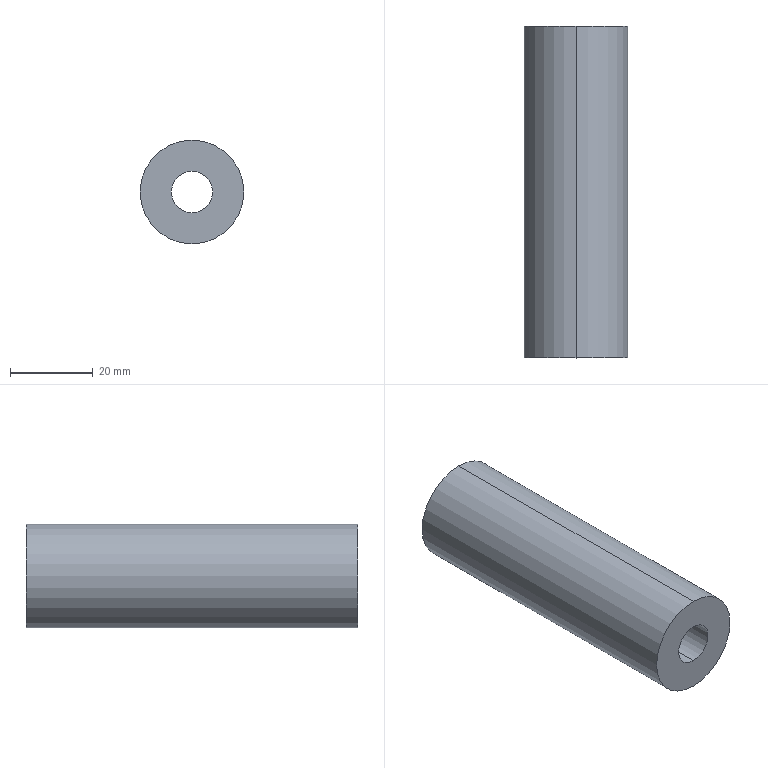Part | STEP file | 1 solid | 6 faces | box 25 x 80 x 25 mm | volume 32987 mm3 | cylinder 4 | plane 2 | commonest cylinder face diameters 10 x2 25 x2
STEP:
#1=CARTESIAN_POINT('',(0.,0.,0.));
#2=DIRECTION('',(0.,0.,1.));
#3=DIRECTION('',(1.,0.,0.));
#4=AXIS2_PLACEMENT_3D('',#1,#2,#3);
#5=CARTESIAN_POINT('',(0.,0.,12.5));
#6=VERTEX_POINT('',#5);
#7=CARTESIAN_POINT('',(0.,0.,-12.5));
#8=VERTEX_POINT('',#7);
#9=CARTESIAN_POINT('',(0.,0.,0.));
#10=DIRECTION('',(0.,1.,0.));
#11=DIRECTION('',(0.,0.,1.));
#12=AXIS2_PLACEMENT_3D('',#9,#10,#11);
#13=CIRCLE('',#12,12.5);
#14=CARTESIAN_POINT('',(0.,0.,0.));
#15=DIRECTION('',(0.,1.,0.));
#16=DIRECTION('',(0.,0.,1.));
#17=AXIS2_PLACEMENT_3D('',#14,#15,#16);
#18=CYLINDRICAL_SURFACE('',#17,12.5);
#19=CARTESIAN_POINT('',(0.,0.));
#20=DIRECTION('',(1.,0.));
#21=VECTOR('',#20,1.);
#22=LINE('',#19,#21);
#23=(GEOMETRIC_REPRESENTATION_CONTEXT(2)PARAMETRIC_REPRESENTATION_CONTEXT()REPRESENTATION_CONTEXT('',''));
#24=DEFINITIONAL_REPRESENTATION('',(#22),#23);
#25=PCURVE('',#18,#24);
#26=CARTESIAN_POINT('',(0.,0.,0.));
#27=DIRECTION('',(0.,1.,0.));
#28=DIRECTION('',(0.,0.,1.));
#29=AXIS2_PLACEMENT_3D('',#26,#27,#28);
#30=PLANE('',#29);
#31=CARTESIAN_POINT('',(0.,0.));
#32=DIRECTION('',(1.,0.));
#33=AXIS2_PLACEMENT_2D('',#31,#32);
#34=CIRCLE('',#33,12.5);
#35=(GEOMETRIC_REPRESENTATION_CONTEXT(2)PARAMETRIC_REPRESENTATION_CONTEXT()REPRESENTATION_CONTEXT('',''));
#36=DEFINITIONAL_REPRESENTATION('',(#34),#35);
#37=PCURVE('',#30,#36);
#38=SURFACE_CURVE('',#13,(#25,#37),.PCURVE_S1.);
#39=EDGE_CURVE('',#6,#8,#38,.T.);
#40=ORIENTED_EDGE('',*,*,#39,.T.);
#41=CARTESIAN_POINT('',(0.,80.,-12.5));
#42=VERTEX_POINT('',#41);
#43=CARTESIAN_POINT('',(0.,0.,-12.5));
#44=DIRECTION('',(0.,1.,0.));
#45=VECTOR('',#44,1.);
#46=LINE('',#43,#45);
#47=CARTESIAN_POINT('',(3.142,0.));
#48=DIRECTION('',(0.,1.));
#49=VECTOR('',#48,1.);
#50=LINE('',#47,#49);
#51=(GEOMETRIC_REPRESENTATION_CONTEXT(2)PARAMETRIC_REPRESENTATION_CONTEXT()REPRESENTATION_CONTEXT('',''));
#52=DEFINITIONAL_REPRESENTATION('',(#50),#51);
#53=PCURVE('',#18,#52);
#54=CARTESIAN_POINT('',(0.,0.,0.));
#55=DIRECTION('',(0.,1.,0.));
#56=DIRECTION('',(0.,0.,1.));
#57=AXIS2_PLACEMENT_3D('',#54,#55,#56);
#58=CYLINDRICAL_SURFACE('',#57,12.5);
#59=CARTESIAN_POINT('',(3.142,0.));
#60=DIRECTION('',(0.,1.));
#61=VECTOR('',#60,1.);
#62=LINE('',#59,#61);
#63=(GEOMETRIC_REPRESENTATION_CONTEXT(2)PARAMETRIC_REPRESENTATION_CONTEXT()REPRESENTATION_CONTEXT('',''));
#64=DEFINITIONAL_REPRESENTATION('',(#62),#63);
#65=PCURVE('',#58,#64);
#66=SURFACE_CURVE('',#46,(#53,#65),.PCURVE_S1.);
#67=EDGE_CURVE('',#8,#42,#66,.T.);
#68=ORIENTED_EDGE('',*,*,#67,.T.);
#69=CARTESIAN_POINT('',(0.,80.,12.5));
#70=VERTEX_POINT('',#69);
#71=CARTESIAN_POINT('',(0.,80.,0.));
#72=DIRECTION('',(0.,-1.,0.));
#73=DIRECTION('',(0.,0.,1.));
#74=AXIS2_PLACEMENT_3D('',#71,#72,#73);
#75=CIRCLE('',#74,12.5);
#76=CARTESIAN_POINT('',(6.283,80.));
#77=DIRECTION('',(-1.,0.));
#78=VECTOR('',#77,1.);
#79=LINE('',#76,#78);
#80=(GEOMETRIC_REPRESENTATION_CONTEXT(2)PARAMETRIC_REPRESENTATION_CONTEXT()REPRESENTATION_CONTEXT('',''));
#81=DEFINITIONAL_REPRESENTATION('',(#79),#80);
#82=PCURVE('',#18,#81);
#83=CARTESIAN_POINT('',(0.,80.,0.));
#84=DIRECTION('',(0.,1.,0.));
#85=DIRECTION('',(0.,0.,1.));
#86=AXIS2_PLACEMENT_3D('',#83,#84,#85);
#87=PLANE('',#86);
#88=CARTESIAN_POINT('',(12.5,0.));
#89=CARTESIAN_POINT('',(12.5,-21.651));
#90=CARTESIAN_POINT('',(-6.25,-10.825));
#91=CARTESIAN_POINT('',(-25.,0.));
#92=CARTESIAN_POINT('',(-6.25,10.825));
#93=CARTESIAN_POINT('',(12.5,21.651));
#94=CARTESIAN_POINT('',(12.5,0.));
#95=(BOUNDED_CURVE()B_SPLINE_CURVE(2,(#88,#89,#90,#91,#92,#93,#94),.UNSPECIFIED.,.T.,.F.)B_SPLINE_CURVE_WITH_KNOTS((1,2,2,2,2,1),(-2.094,0.,2.094,4.189,6.283,8.378),.UNSPECIFIED.)CURVE()GEOMETRIC_REPRESENTATION_ITEM()RATIONAL_B_SPLINE_CURVE((1.,0.5,1.,0.5,1.,0.5,1.))REPRESENTATION_ITEM(''));
#96=(GEOMETRIC_REPRESENTATION_CONTEXT(2)PARAMETRIC_REPRESENTATION_CONTEXT()REPRESENTATION_CONTEXT('',''));
#97=DEFINITIONAL_REPRESENTATION('',(#95),#96);
#98=PCURVE('',#87,#97);
#99=SURFACE_CURVE('',#75,(#82,#98),.PCURVE_S1.);
#100=EDGE_CURVE('',#42,#70,#99,.T.);
#101=ORIENTED_EDGE('',*,*,#100,.T.);
#102=CARTESIAN_POINT('',(0.,0.,12.5));
#103=DIRECTION('',(0.,1.,0.));
#104=VECTOR('',#103,1.);
#105=LINE('',#102,#104);
#106=CARTESIAN_POINT('',(0.,0.));
#107=DIRECTION('',(0.,1.));
#108=VECTOR('',#107,1.);
#109=LINE('',#106,#108);
#110=(GEOMETRIC_REPRESENTATION_CONTEXT(2)PARAMETRIC_REPRESENTATION_CONTEXT()REPRESENTATION_CONTEXT('',''));
#111=DEFINITIONAL_REPRESENTATION('',(#109),#110);
#112=PCURVE('',#18,#111);
#113=CARTESIAN_POINT('',(6.283,0.));
#114=DIRECTION('',(0.,1.));
#115=VECTOR('',#114,1.);
#116=LINE('',#113,#115);
#117=(GEOMETRIC_REPRESENTATION_CONTEXT(2)PARAMETRIC_REPRESENTATION_CONTEXT()REPRESENTATION_CONTEXT('',''));
#118=DEFINITIONAL_REPRESENTATION('',(#116),#117);
#119=PCURVE('',#58,#118);
#120=SURFACE_CURVE('',#105,(#112,#119),.PCURVE_S1.);
#121=EDGE_CURVE('',#6,#70,#120,.T.);
#122=ORIENTED_EDGE('',*,*,#121,.F.);
#123=EDGE_LOOP('',(#40,#68,#101,#122));
#124=FACE_BOUND('',#123,.T.);
#125=ADVANCED_FACE('',(#124),#18,.T.);
#126=CARTESIAN_POINT('',(0.,0.,5.));
#127=VERTEX_POINT('',#126);
#128=CARTESIAN_POINT('',(0.,80.,5.));
#129=VERTEX_POINT('',#128);
#130=CARTESIAN_POINT('',(0.,0.,5.));
#131=DIRECTION('',(0.,1.,0.));
#132=VECTOR('',#131,1.);
#133=LINE('',#130,#132);
#134=CARTESIAN_POINT('',(0.,0.,0.));
#135=DIRECTION('',(0.,1.,0.));
#136=DIRECTION('',(0.,0.,1.));
#137=AXIS2_PLACEMENT_3D('',#134,#135,#136);
#138=CYLINDRICAL_SURFACE('',#137,5.);
#139=CARTESIAN_POINT('',(6.283,0.));
#140=DIRECTION('',(0.,1.));
#141=VECTOR('',#140,1.);
#142=LINE('',#139,#141);
#143=(GEOMETRIC_REPRESENTATION_CONTEXT(2)PARAMETRIC_REPRESENTATION_CONTEXT()REPRESENTATION_CONTEXT('',''));
#144=DEFINITIONAL_REPRESENTATION('',(#142),#143);
#145=PCURVE('',#138,#144);
#146=CARTESIAN_POINT('',(0.,0.,0.));
#147=DIRECTION('',(0.,1.,0.));
#148=DIRECTION('',(0.,0.,1.));
#149=AXIS2_PLACEMENT_3D('',#146,#147,#148);
#150=CYLINDRICAL_SURFACE('',#149,5.);
#151=CARTESIAN_POINT('',(0.,0.));
#152=DIRECTION('',(0.,1.));
#153=VECTOR('',#152,1.);
#154=LINE('',#151,#153);
#155=(GEOMETRIC_REPRESENTATION_CONTEXT(2)PARAMETRIC_REPRESENTATION_CONTEXT()REPRESENTATION_CONTEXT('',''));
#156=DEFINITIONAL_REPRESENTATION('',(#154),#155);
#157=PCURVE('',#150,#156);
#158=SURFACE_CURVE('',#133,(#145,#157),.PCURVE_S1.);
#159=EDGE_CURVE('',#127,#129,#158,.T.);
#160=ORIENTED_EDGE('',*,*,#159,.T.);
#161=CARTESIAN_POINT('',(0.,80.,-5.));
#162=VERTEX_POINT('',#161);
#163=CARTESIAN_POINT('',(0.,80.,0.));
#164=DIRECTION('',(0.,-1.,0.));
#165=DIRECTION('',(0.,0.,1.));
#166=AXIS2_PLACEMENT_3D('',#163,#164,#165);
#167=CIRCLE('',#166,5.);
#168=CARTESIAN_POINT('',(6.283,80.));
#169=DIRECTION('',(-1.,0.));
#170=VECTOR('',#169,1.);
#171=LINE('',#168,#170);
#172=(GEOMETRIC_REPRESENTATION_CONTEXT(2)PARAMETRIC_REPRESENTATION_CONTEXT()REPRESENTATION_CONTEXT('',''));
#173=DEFINITIONAL_REPRESENTATION('',(#171),#172);
#174=PCURVE('',#138,#173);
#175=CARTESIAN_POINT('',(5.,0.));
#176=CARTESIAN_POINT('',(5.,-8.66));
#177=CARTESIAN_POINT('',(-2.5,-4.33));
#178=CARTESIAN_POINT('',(-10.,0.));
#179=CARTESIAN_POINT('',(-2.5,4.33));
#180=CARTESIAN_POINT('',(5.,8.66));
#181=CARTESIAN_POINT('',(5.,0.));
#182=(BOUNDED_CURVE()B_SPLINE_CURVE(2,(#175,#176,#177,#178,#179,#180,#181),.UNSPECIFIED.,.T.,.F.)B_SPLINE_CURVE_WITH_KNOTS((1,2,2,2,2,1),(-2.094,0.,2.094,4.189,6.283,8.378),.UNSPECIFIED.)CURVE()GEOMETRIC_REPRESENTATION_ITEM()RATIONAL_B_SPLINE_CURVE((1.,0.5,1.,0.5,1.,0.5,1.))REPRESENTATION_ITEM(''));
#183=(GEOMETRIC_REPRESENTATION_CONTEXT(2)PARAMETRIC_REPRESENTATION_CONTEXT()REPRESENTATION_CONTEXT('',''));
#184=DEFINITIONAL_REPRESENTATION('',(#182),#183);
#185=PCURVE('',#87,#184);
#186=SURFACE_CURVE('',#167,(#174,#185),.PCURVE_S1.);
#187=EDGE_CURVE('',#129,#162,#186,.T.);
#188=ORIENTED_EDGE('',*,*,#187,.T.);
#189=CARTESIAN_POINT('',(0.,0.,-5.));
#190=VERTEX_POINT('',#189);
#191=CARTESIAN_POINT('',(0.,0.,-5.));
#192=DIRECTION('',(0.,1.,0.));
#193=VECTOR('',#192,1.);
#194=LINE('',#191,#193);
#195=CARTESIAN_POINT('',(3.142,0.));
#196=DIRECTION('',(0.,1.));
#197=VECTOR('',#196,1.);
#198=LINE('',#195,#197);
#199=(GEOMETRIC_REPRESENTATION_CONTEXT(2)PARAMETRIC_REPRESENTATION_CONTEXT()REPRESENTATION_CONTEXT('',''));
#200=DEFINITIONAL_REPRESENTATION('',(#198),#199);
#201=PCURVE('',#138,#200);
#202=CARTESIAN_POINT('',(3.142,0.));
#203=DIRECTION('',(0.,1.));
#204=VECTOR('',#203,1.);
#205=LINE('',#202,#204);
#206=(GEOMETRIC_REPRESENTATION_CONTEXT(2)PARAMETRIC_REPRESENTATION_CONTEXT()REPRESENTATION_CONTEXT('',''));
#207=DEFINITIONAL_REPRESENTATION('',(#205),#206);
#208=PCURVE('',#150,#207);
#209=SURFACE_CURVE('',#194,(#201,#208),.PCURVE_S1.);
#210=EDGE_CURVE('',#190,#162,#209,.T.);
#211=ORIENTED_EDGE('',*,*,#210,.F.);
#212=CARTESIAN_POINT('',(0.,0.,0.));
#213=DIRECTION('',(0.,-1.,0.));
#214=DIRECTION('',(0.,0.,1.));
#215=AXIS2_PLACEMENT_3D('',#212,#213,#214);
#216=CIRCLE('',#215,5.);
#217=CARTESIAN_POINT('',(6.283,0.));
#218=DIRECTION('',(-1.,0.));
#219=VECTOR('',#218,1.);
#220=LINE('',#217,#219);
#221=(GEOMETRIC_REPRESENTATION_CONTEXT(2)PARAMETRIC_REPRESENTATION_CONTEXT()REPRESENTATION_CONTEXT('',''));
#222=DEFINITIONAL_REPRESENTATION('',(#220),#221);
#223=PCURVE('',#138,#222);
#224=CARTESIAN_POINT('',(5.,0.));
#225=CARTESIAN_POINT('',(5.,-8.66));
#226=CARTESIAN_POINT('',(-2.5,-4.33));
#227=CARTESIAN_POINT('',(-10.,0.));
#228=CARTESIAN_POINT('',(-2.5,4.33));
#229=CARTESIAN_POINT('',(5.,8.66));
#230=CARTESIAN_POINT('',(5.,0.));
#231=(BOUNDED_CURVE()B_SPLINE_CURVE(2,(#224,#225,#226,#227,#228,#229,#230),.UNSPECIFIED.,.T.,.F.)B_SPLINE_CURVE_WITH_KNOTS((1,2,2,2,2,1),(-2.094,0.,2.094,4.189,6.283,8.378),.UNSPECIFIED.)CURVE()GEOMETRIC_REPRESENTATION_ITEM()RATIONAL_B_SPLINE_CURVE((1.,0.5,1.,0.5,1.,0.5,1.))REPRESENTATION_ITEM(''));
#232=(GEOMETRIC_REPRESENTATION_CONTEXT(2)PARAMETRIC_REPRESENTATION_CONTEXT()REPRESENTATION_CONTEXT('',''));
#233=DEFINITIONAL_REPRESENTATION('',(#231),#232);
#234=PCURVE('',#30,#233);
#235=SURFACE_CURVE('',#216,(#223,#234),.PCURVE_S1.);
#236=EDGE_CURVE('',#127,#190,#235,.T.);
#237=ORIENTED_EDGE('',*,*,#236,.F.);
#238=EDGE_LOOP('',(#160,#188,#211,#237));
#239=FACE_BOUND('',#238,.F.);
#240=ADVANCED_FACE('',(#239),#138,.F.);
#241=ORIENTED_EDGE('',*,*,#67,.F.);
#242=CARTESIAN_POINT('',(0.,0.,0.));
#243=DIRECTION('',(0.,1.,0.));
#244=DIRECTION('',(0.,0.,1.));
#245=AXIS2_PLACEMENT_3D('',#242,#243,#244);
#246=CIRCLE('',#245,12.5);
#247=CARTESIAN_POINT('',(0.,0.));
#248=DIRECTION('',(1.,0.));
#249=VECTOR('',#248,1.);
#250=LINE('',#247,#249);
#251=(GEOMETRIC_REPRESENTATION_CONTEXT(2)PARAMETRIC_REPRESENTATION_CONTEXT()REPRESENTATION_CONTEXT('',''));
#252=DEFINITIONAL_REPRESENTATION('',(#250),#251);
#253=PCURVE('',#58,#252);
#254=CARTESIAN_POINT('',(0.,0.));
#255=DIRECTION('',(1.,0.));
#256=AXIS2_PLACEMENT_2D('',#254,#255);
#257=CIRCLE('',#256,12.5);
#258=(GEOMETRIC_REPRESENTATION_CONTEXT(2)PARAMETRIC_REPRESENTATION_CONTEXT()REPRESENTATION_CONTEXT('',''));
#259=DEFINITIONAL_REPRESENTATION('',(#257),#258);
#260=PCURVE('',#30,#259);
#261=SURFACE_CURVE('',#246,(#253,#260),.PCURVE_S1.);
#262=EDGE_CURVE('',#8,#6,#261,.T.);
#263=ORIENTED_EDGE('',*,*,#262,.T.);
#264=ORIENTED_EDGE('',*,*,#121,.T.);
#265=CARTESIAN_POINT('',(0.,80.,0.));
#266=DIRECTION('',(0.,-1.,0.));
#267=DIRECTION('',(0.,0.,1.));
#268=AXIS2_PLACEMENT_3D('',#265,#266,#267);
#269=CIRCLE('',#268,12.5);
#270=CARTESIAN_POINT('',(6.283,80.));
#271=DIRECTION('',(-1.,0.));
#272=VECTOR('',#271,1.);
#273=LINE('',#270,#272);
#274=(GEOMETRIC_REPRESENTATION_CONTEXT(2)PARAMETRIC_REPRESENTATION_CONTEXT()REPRESENTATION_CONTEXT('',''));
#275=DEFINITIONAL_REPRESENTATION('',(#273),#274);
#276=PCURVE('',#58,#275);
#277=CARTESIAN_POINT('',(12.5,0.));
#278=CARTESIAN_POINT('',(12.5,-21.651));
#279=CARTESIAN_POINT('',(-6.25,-10.825));
#280=CARTESIAN_POINT('',(-25.,0.));
#281=CARTESIAN_POINT('',(-6.25,10.825));
#282=CARTESIAN_POINT('',(12.5,21.651));
#283=CARTESIAN_POINT('',(12.5,0.));
#284=(BOUNDED_CURVE()B_SPLINE_CURVE(2,(#277,#278,#279,#280,#281,#282,#283),.UNSPECIFIED.,.T.,.F.)B_SPLINE_CURVE_WITH_KNOTS((1,2,2,2,2,1),(-2.094,0.,2.094,4.189,6.283,8.378),.UNSPECIFIED.)CURVE()GEOMETRIC_REPRESENTATION_ITEM()RATIONAL_B_SPLINE_CURVE((1.,0.5,1.,0.5,1.,0.5,1.))REPRESENTATION_ITEM(''));
#285=(GEOMETRIC_REPRESENTATION_CONTEXT(2)PARAMETRIC_REPRESENTATION_CONTEXT()REPRESENTATION_CONTEXT('',''));
#286=DEFINITIONAL_REPRESENTATION('',(#284),#285);
#287=PCURVE('',#87,#286);
#288=SURFACE_CURVE('',#269,(#276,#287),.PCURVE_S1.);
#289=EDGE_CURVE('',#70,#42,#288,.T.);
#290=ORIENTED_EDGE('',*,*,#289,.T.);
#291=EDGE_LOOP('',(#241,#263,#264,#290));
#292=FACE_BOUND('',#291,.T.);
#293=ADVANCED_FACE('',(#292),#58,.T.);
#294=ORIENTED_EDGE('',*,*,#39,.F.);
#295=ORIENTED_EDGE('',*,*,#262,.F.);
#296=EDGE_LOOP('',(#294,#295));
#297=FACE_BOUND('',#296,.T.);
#298=ORIENTED_EDGE('',*,*,#236,.F.);
#299=CARTESIAN_POINT('',(0.,0.,0.));
#300=DIRECTION('',(0.,-1.,0.));
#301=DIRECTION('',(0.,0.,1.));
#302=AXIS2_PLACEMENT_3D('',#299,#300,#301);
#303=CIRCLE('',#302,5.);
#304=CARTESIAN_POINT('',(5.,0.));
#305=CARTESIAN_POINT('',(5.,-8.66));
#306=CARTESIAN_POINT('',(-2.5,-4.33));
#307=CARTESIAN_POINT('',(-10.,0.));
#308=CARTESIAN_POINT('',(-2.5,4.33));
#309=CARTESIAN_POINT('',(5.,8.66));
#310=CARTESIAN_POINT('',(5.,0.));
#311=(BOUNDED_CURVE()B_SPLINE_CURVE(2,(#304,#305,#306,#307,#308,#309,#310),.UNSPECIFIED.,.T.,.F.)B_SPLINE_CURVE_WITH_KNOTS((1,2,2,2,2,1),(-2.094,0.,2.094,4.189,6.283,8.378),.UNSPECIFIED.)CURVE()GEOMETRIC_REPRESENTATION_ITEM()RATIONAL_B_SPLINE_CURVE((1.,0.5,1.,0.5,1.,0.5,1.))REPRESENTATION_ITEM(''));
#312=(GEOMETRIC_REPRESENTATION_CONTEXT(2)PARAMETRIC_REPRESENTATION_CONTEXT()REPRESENTATION_CONTEXT('',''));
#313=DEFINITIONAL_REPRESENTATION('',(#311),#312);
#314=PCURVE('',#30,#313);
#315=CARTESIAN_POINT('',(6.283,0.));
#316=DIRECTION('',(-1.,0.));
#317=VECTOR('',#316,1.);
#318=LINE('',#315,#317);
#319=(GEOMETRIC_REPRESENTATION_CONTEXT(2)PARAMETRIC_REPRESENTATION_CONTEXT()REPRESENTATION_CONTEXT('',''));
#320=DEFINITIONAL_REPRESENTATION('',(#318),#319);
#321=PCURVE('',#150,#320);
#322=SURFACE_CURVE('',#303,(#314,#321),.PCURVE_S1.);
#323=EDGE_CURVE('',#190,#127,#322,.T.);
#324=ORIENTED_EDGE('',*,*,#323,.F.);
#325=EDGE_LOOP('',(#298,#324));
#326=FACE_BOUND('',#325,.T.);
#327=ADVANCED_FACE('',(#297,#326),#30,.F.);
#328=ORIENTED_EDGE('',*,*,#289,.F.);
#329=ORIENTED_EDGE('',*,*,#100,.F.);
#330=EDGE_LOOP('',(#328,#329));
#331=FACE_BOUND('',#330,.T.);
#332=ORIENTED_EDGE('',*,*,#187,.T.);
#333=CARTESIAN_POINT('',(0.,80.,0.));
#334=DIRECTION('',(0.,-1.,0.));
#335=DIRECTION('',(0.,0.,1.));
#336=AXIS2_PLACEMENT_3D('',#333,#334,#335);
#337=CIRCLE('',#336,5.);
#338=CARTESIAN_POINT('',(5.,0.));
#339=CARTESIAN_POINT('',(5.,-8.66));
#340=CARTESIAN_POINT('',(-2.5,-4.33));
#341=CARTESIAN_POINT('',(-10.,0.));
#342=CARTESIAN_POINT('',(-2.5,4.33));
#343=CARTESIAN_POINT('',(5.,8.66));
#344=CARTESIAN_POINT('',(5.,0.));
#345=(BOUNDED_CURVE()B_SPLINE_CURVE(2,(#338,#339,#340,#341,#342,#343,#344),.UNSPECIFIED.,.T.,.F.)B_SPLINE_CURVE_WITH_KNOTS((1,2,2,2,2,1),(-2.094,0.,2.094,4.189,6.283,8.378),.UNSPECIFIED.)CURVE()GEOMETRIC_REPRESENTATION_ITEM()RATIONAL_B_SPLINE_CURVE((1.,0.5,1.,0.5,1.,0.5,1.))REPRESENTATION_ITEM(''));
#346=(GEOMETRIC_REPRESENTATION_CONTEXT(2)PARAMETRIC_REPRESENTATION_CONTEXT()REPRESENTATION_CONTEXT('',''));
#347=DEFINITIONAL_REPRESENTATION('',(#345),#346);
#348=PCURVE('',#87,#347);
#349=CARTESIAN_POINT('',(6.283,80.));
#350=DIRECTION('',(-1.,0.));
#351=VECTOR('',#350,1.);
#352=LINE('',#349,#351);
#353=(GEOMETRIC_REPRESENTATION_CONTEXT(2)PARAMETRIC_REPRESENTATION_CONTEXT()REPRESENTATION_CONTEXT('',''));
#354=DEFINITIONAL_REPRESENTATION('',(#352),#353);
#355=PCURVE('',#150,#354);
#356=SURFACE_CURVE('',#337,(#348,#355),.PCURVE_S1.);
#357=EDGE_CURVE('',#162,#129,#356,.T.);
#358=ORIENTED_EDGE('',*,*,#357,.T.);
#359=EDGE_LOOP('',(#332,#358));
#360=FACE_BOUND('',#359,.T.);
#361=ADVANCED_FACE('',(#331,#360),#87,.T.);
#362=ORIENTED_EDGE('',*,*,#357,.T.);
#363=ORIENTED_EDGE('',*,*,#159,.F.);
#364=ORIENTED_EDGE('',*,*,#323,.F.);
#365=ORIENTED_EDGE('',*,*,#210,.T.);
#366=EDGE_LOOP('',(#362,#363,#364,#365));
#367=FACE_BOUND('',#366,.F.);
#368=ADVANCED_FACE('',(#367),#150,.F.);
#369=CLOSED_SHELL('',(#125,#240,#293,#327,#361,#368));
#370=MANIFOLD_SOLID_BREP('',#369);
#371=(LENGTH_UNIT()NAMED_UNIT(*)SI_UNIT(.MILLI.,.METRE.));
#372=UNCERTAINTY_MEASURE_WITH_UNIT(LENGTH_MEASURE(0.0000001),#371,'','');
#373=(NAMED_UNIT(*)PLANE_ANGLE_UNIT()SI_UNIT($,.RADIAN.));
#374=(NAMED_UNIT(*)SI_UNIT($,.STERADIAN.)SOLID_ANGLE_UNIT());
#375=(GEOMETRIC_REPRESENTATION_CONTEXT(3)GLOBAL_UNCERTAINTY_ASSIGNED_CONTEXT((#372))GLOBAL_UNIT_ASSIGNED_CONTEXT((#371,#373,#374))REPRESENTATION_CONTEXT('',''));
#376=ADVANCED_BREP_SHAPE_REPRESENTATION('',(#4,#370),#375);